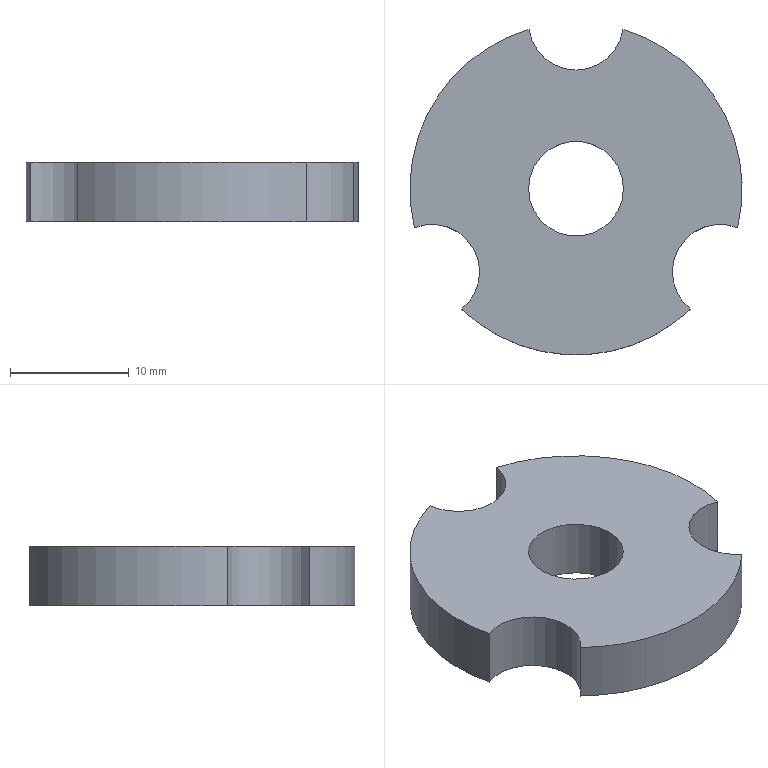Part | STEP file | PN_0002_default | 1 solid | 9 faces | box 28 x 27.429 x 5 mm | volume 2473 mm3 | cylinder 7 | plane 2 | commonest cylinder face diameters 8 x4 28 x3
STEP:
#1=CARTESIAN_POINT('',(0.,0.,0.));
#2=DIRECTION('',(0.,0.,1.));
#3=DIRECTION('',(1.,0.,0.));
#4=AXIS2_PLACEMENT_3D('',#1,#2,#3);
#5=CARTESIAN_POINT('',(-9.65,-10.143,5.));
#6=VERTEX_POINT('',#5);
#7=CARTESIAN_POINT('',(9.65,-10.143,5.));
#8=VERTEX_POINT('',#7);
#9=CARTESIAN_POINT('',(0.,0.,5.));
#10=DIRECTION('',(0.,0.,1.));
#11=DIRECTION('',(1.,0.,0.));
#12=AXIS2_PLACEMENT_3D('',#9,#10,#11);
#13=CIRCLE('',#12,14.);
#14=CARTESIAN_POINT('',(6.062,-3.5,5.));
#15=DIRECTION('',(0.,0.,1.));
#16=DIRECTION('',(1.,0.,0.));
#17=AXIS2_PLACEMENT_3D('',#14,#15,#16);
#18=PLANE('',#17);
#19=CARTESIAN_POINT('',(-6.062,3.5));
#20=DIRECTION('',(1.,0.));
#21=AXIS2_PLACEMENT_2D('',#19,#20);
#22=CIRCLE('',#21,14.);
#23=(GEOMETRIC_REPRESENTATION_CONTEXT(2)PARAMETRIC_REPRESENTATION_CONTEXT()REPRESENTATION_CONTEXT('',''));
#24=DEFINITIONAL_REPRESENTATION('',(#22),#23);
#25=PCURVE('',#18,#24);
#26=CARTESIAN_POINT('',(0.,0.,5.));
#27=DIRECTION('',(0.,0.,-1.));
#28=DIRECTION('',(-1.,0.,0.));
#29=AXIS2_PLACEMENT_3D('',#26,#27,#28);
#30=CYLINDRICAL_SURFACE('',#29,14.);
#31=CARTESIAN_POINT('',(9.425,0.));
#32=DIRECTION('',(-1.,0.));
#33=VECTOR('',#32,1.);
#34=LINE('',#31,#33);
#35=(GEOMETRIC_REPRESENTATION_CONTEXT(2)PARAMETRIC_REPRESENTATION_CONTEXT()REPRESENTATION_CONTEXT('',''));
#36=DEFINITIONAL_REPRESENTATION('',(#34),#35);
#37=PCURVE('',#30,#36);
#38=SURFACE_CURVE('',#13,(#25,#37),.PCURVE_S1.);
#39=EDGE_CURVE('',#6,#8,#38,.T.);
#40=ORIENTED_EDGE('',*,*,#39,.T.);
#41=CARTESIAN_POINT('',(13.609,-3.286,5.));
#42=VERTEX_POINT('',#41);
#43=CARTESIAN_POINT('',(12.124,-7.,5.));
#44=DIRECTION('',(0.,0.,-1.));
#45=DIRECTION('',(1.,0.,0.));
#46=AXIS2_PLACEMENT_3D('',#43,#44,#45);
#47=CIRCLE('',#46,4.);
#48=CARTESIAN_POINT('',(10.062,-3.5));
#49=CARTESIAN_POINT('',(10.062,-10.428));
#50=CARTESIAN_POINT('',(4.062,-6.964));
#51=CARTESIAN_POINT('',(-1.938,-3.5));
#52=CARTESIAN_POINT('',(4.062,-0.0359));
#53=CARTESIAN_POINT('',(10.062,3.428));
#54=CARTESIAN_POINT('',(10.062,-3.5));
#55=(BOUNDED_CURVE()B_SPLINE_CURVE(2,(#48,#49,#50,#51,#52,#53,#54),.UNSPECIFIED.,.T.,.F.)B_SPLINE_CURVE_WITH_KNOTS((1,2,2,2,2,1),(-2.094,0.,2.094,4.189,6.283,8.378),.UNSPECIFIED.)CURVE()GEOMETRIC_REPRESENTATION_ITEM()RATIONAL_B_SPLINE_CURVE((1.,0.5,1.,0.5,1.,0.5,1.))REPRESENTATION_ITEM(''));
#56=(GEOMETRIC_REPRESENTATION_CONTEXT(2)PARAMETRIC_REPRESENTATION_CONTEXT()REPRESENTATION_CONTEXT('',''));
#57=DEFINITIONAL_REPRESENTATION('',(#55),#56);
#58=PCURVE('',#18,#57);
#59=CARTESIAN_POINT('',(12.124,-7.,5.));
#60=DIRECTION('',(0.,0.,-1.));
#61=DIRECTION('',(-1.,0.,0.));
#62=AXIS2_PLACEMENT_3D('',#59,#60,#61);
#63=CYLINDRICAL_SURFACE('',#62,4.);
#64=CARTESIAN_POINT('',(-3.142,0.));
#65=DIRECTION('',(1.,0.));
#66=VECTOR('',#65,1.);
#67=LINE('',#64,#66);
#68=(GEOMETRIC_REPRESENTATION_CONTEXT(2)PARAMETRIC_REPRESENTATION_CONTEXT()REPRESENTATION_CONTEXT('',''));
#69=DEFINITIONAL_REPRESENTATION('',(#67),#68);
#70=PCURVE('',#63,#69);
#71=SURFACE_CURVE('',#47,(#58,#70),.PCURVE_S1.);
#72=EDGE_CURVE('',#8,#42,#71,.T.);
#73=ORIENTED_EDGE('',*,*,#72,.T.);
#74=CARTESIAN_POINT('',(3.959,13.429,5.));
#75=VERTEX_POINT('',#74);
#76=CARTESIAN_POINT('',(0.,0.,5.));
#77=DIRECTION('',(0.,0.,1.));
#78=DIRECTION('',(1.,0.,0.));
#79=AXIS2_PLACEMENT_3D('',#76,#77,#78);
#80=CIRCLE('',#79,14.);
#81=CARTESIAN_POINT('',(-6.062,3.5));
#82=DIRECTION('',(1.,0.));
#83=AXIS2_PLACEMENT_2D('',#81,#82);
#84=CIRCLE('',#83,14.);
#85=(GEOMETRIC_REPRESENTATION_CONTEXT(2)PARAMETRIC_REPRESENTATION_CONTEXT()REPRESENTATION_CONTEXT('',''));
#86=DEFINITIONAL_REPRESENTATION('',(#84),#85);
#87=PCURVE('',#18,#86);
#88=CARTESIAN_POINT('',(0.,0.,5.));
#89=DIRECTION('',(0.,0.,-1.));
#90=DIRECTION('',(-1.,0.,0.));
#91=AXIS2_PLACEMENT_3D('',#88,#89,#90);
#92=CYLINDRICAL_SURFACE('',#91,14.);
#93=CARTESIAN_POINT('',(9.425,0.));
#94=DIRECTION('',(-1.,0.));
#95=VECTOR('',#94,1.);
#96=LINE('',#93,#95);
#97=(GEOMETRIC_REPRESENTATION_CONTEXT(2)PARAMETRIC_REPRESENTATION_CONTEXT()REPRESENTATION_CONTEXT('',''));
#98=DEFINITIONAL_REPRESENTATION('',(#96),#97);
#99=PCURVE('',#92,#98);
#100=SURFACE_CURVE('',#80,(#87,#99),.PCURVE_S1.);
#101=EDGE_CURVE('',#42,#75,#100,.T.);
#102=ORIENTED_EDGE('',*,*,#101,.T.);
#103=CARTESIAN_POINT('',(-3.959,13.429,5.));
#104=VERTEX_POINT('',#103);
#105=CARTESIAN_POINT('',(0.,14.,5.));
#106=DIRECTION('',(0.,0.,-1.));
#107=DIRECTION('',(1.,0.,0.));
#108=AXIS2_PLACEMENT_3D('',#105,#106,#107);
#109=CIRCLE('',#108,4.);
#110=CARTESIAN_POINT('',(-2.062,17.5));
#111=CARTESIAN_POINT('',(-2.062,10.572));
#112=CARTESIAN_POINT('',(-8.062,14.036));
#113=CARTESIAN_POINT('',(-14.062,17.5));
#114=CARTESIAN_POINT('',(-8.062,20.964));
#115=CARTESIAN_POINT('',(-2.062,24.428));
#116=CARTESIAN_POINT('',(-2.062,17.5));
#117=(BOUNDED_CURVE()B_SPLINE_CURVE(2,(#110,#111,#112,#113,#114,#115,#116),.UNSPECIFIED.,.T.,.F.)B_SPLINE_CURVE_WITH_KNOTS((1,2,2,2,2,1),(-2.094,0.,2.094,4.189,6.283,8.378),.UNSPECIFIED.)CURVE()GEOMETRIC_REPRESENTATION_ITEM()RATIONAL_B_SPLINE_CURVE((1.,0.5,1.,0.5,1.,0.5,1.))REPRESENTATION_ITEM(''));
#118=(GEOMETRIC_REPRESENTATION_CONTEXT(2)PARAMETRIC_REPRESENTATION_CONTEXT()REPRESENTATION_CONTEXT('',''));
#119=DEFINITIONAL_REPRESENTATION('',(#117),#118);
#120=PCURVE('',#18,#119);
#121=CARTESIAN_POINT('',(0.,14.,5.));
#122=DIRECTION('',(0.,0.,-1.));
#123=DIRECTION('',(-1.,0.,0.));
#124=AXIS2_PLACEMENT_3D('',#121,#122,#123);
#125=CYLINDRICAL_SURFACE('',#124,4.);
#126=CARTESIAN_POINT('',(3.142,0.));
#127=DIRECTION('',(1.,0.));
#128=VECTOR('',#127,1.);
#129=LINE('',#126,#128);
#130=(GEOMETRIC_REPRESENTATION_CONTEXT(2)PARAMETRIC_REPRESENTATION_CONTEXT()REPRESENTATION_CONTEXT('',''));
#131=DEFINITIONAL_REPRESENTATION('',(#129),#130);
#132=PCURVE('',#125,#131);
#133=SURFACE_CURVE('',#109,(#120,#132),.PCURVE_S1.);
#134=EDGE_CURVE('',#75,#104,#133,.T.);
#135=ORIENTED_EDGE('',*,*,#134,.T.);
#136=CARTESIAN_POINT('',(-13.609,-3.286,5.));
#137=VERTEX_POINT('',#136);
#138=CARTESIAN_POINT('',(0.,0.,5.));
#139=DIRECTION('',(0.,0.,1.));
#140=DIRECTION('',(1.,0.,0.));
#141=AXIS2_PLACEMENT_3D('',#138,#139,#140);
#142=CIRCLE('',#141,14.);
#143=CARTESIAN_POINT('',(-6.062,3.5));
#144=DIRECTION('',(1.,0.));
#145=AXIS2_PLACEMENT_2D('',#143,#144);
#146=CIRCLE('',#145,14.);
#147=(GEOMETRIC_REPRESENTATION_CONTEXT(2)PARAMETRIC_REPRESENTATION_CONTEXT()REPRESENTATION_CONTEXT('',''));
#148=DEFINITIONAL_REPRESENTATION('',(#146),#147);
#149=PCURVE('',#18,#148);
#150=CARTESIAN_POINT('',(0.,0.,5.));
#151=DIRECTION('',(0.,0.,-1.));
#152=DIRECTION('',(-1.,0.,0.));
#153=AXIS2_PLACEMENT_3D('',#150,#151,#152);
#154=CYLINDRICAL_SURFACE('',#153,14.);
#155=CARTESIAN_POINT('',(3.142,0.));
#156=DIRECTION('',(-1.,0.));
#157=VECTOR('',#156,1.);
#158=LINE('',#155,#157);
#159=(GEOMETRIC_REPRESENTATION_CONTEXT(2)PARAMETRIC_REPRESENTATION_CONTEXT()REPRESENTATION_CONTEXT('',''));
#160=DEFINITIONAL_REPRESENTATION('',(#158),#159);
#161=PCURVE('',#154,#160);
#162=SURFACE_CURVE('',#142,(#149,#161),.PCURVE_S1.);
#163=EDGE_CURVE('',#104,#137,#162,.T.);
#164=ORIENTED_EDGE('',*,*,#163,.T.);
#165=CARTESIAN_POINT('',(-12.124,-7.,5.));
#166=DIRECTION('',(0.,0.,-1.));
#167=DIRECTION('',(1.,0.,0.));
#168=AXIS2_PLACEMENT_3D('',#165,#166,#167);
#169=CIRCLE('',#168,4.);
#170=CARTESIAN_POINT('',(-14.187,-3.5));
#171=CARTESIAN_POINT('',(-14.187,-10.428));
#172=CARTESIAN_POINT('',(-20.187,-6.964));
#173=CARTESIAN_POINT('',(-26.187,-3.5));
#174=CARTESIAN_POINT('',(-20.187,-0.0359));
#175=CARTESIAN_POINT('',(-14.187,3.428));
#176=CARTESIAN_POINT('',(-14.187,-3.5));
#177=(BOUNDED_CURVE()B_SPLINE_CURVE(2,(#170,#171,#172,#173,#174,#175,#176),.UNSPECIFIED.,.T.,.F.)B_SPLINE_CURVE_WITH_KNOTS((1,2,2,2,2,1),(-2.094,0.,2.094,4.189,6.283,8.378),.UNSPECIFIED.)CURVE()GEOMETRIC_REPRESENTATION_ITEM()RATIONAL_B_SPLINE_CURVE((1.,0.5,1.,0.5,1.,0.5,1.))REPRESENTATION_ITEM(''));
#178=(GEOMETRIC_REPRESENTATION_CONTEXT(2)PARAMETRIC_REPRESENTATION_CONTEXT()REPRESENTATION_CONTEXT('',''));
#179=DEFINITIONAL_REPRESENTATION('',(#177),#178);
#180=PCURVE('',#18,#179);
#181=CARTESIAN_POINT('',(-12.124,-7.,5.));
#182=DIRECTION('',(0.,0.,-1.));
#183=DIRECTION('',(-1.,0.,0.));
#184=AXIS2_PLACEMENT_3D('',#181,#182,#183);
#185=CYLINDRICAL_SURFACE('',#184,4.);
#186=CARTESIAN_POINT('',(-3.142,0.));
#187=DIRECTION('',(1.,0.));
#188=VECTOR('',#187,1.);
#189=LINE('',#186,#188);
#190=(GEOMETRIC_REPRESENTATION_CONTEXT(2)PARAMETRIC_REPRESENTATION_CONTEXT()REPRESENTATION_CONTEXT('',''));
#191=DEFINITIONAL_REPRESENTATION('',(#189),#190);
#192=PCURVE('',#185,#191);
#193=SURFACE_CURVE('',#169,(#180,#192),.PCURVE_S1.);
#194=EDGE_CURVE('',#137,#6,#193,.T.);
#195=ORIENTED_EDGE('',*,*,#194,.T.);
#196=EDGE_LOOP('',(#40,#73,#102,#135,#164,#195));
#197=FACE_BOUND('',#196,.T.);
#198=CARTESIAN_POINT('',(4.,0.,5.));
#199=VERTEX_POINT('',#198);
#200=CARTESIAN_POINT('',(0.,0.,5.));
#201=DIRECTION('',(0.,0.,1.));
#202=DIRECTION('',(1.,0.,0.));
#203=AXIS2_PLACEMENT_3D('',#200,#201,#202);
#204=CIRCLE('',#203,4.);
#205=CARTESIAN_POINT('',(-6.062,3.5));
#206=DIRECTION('',(1.,0.));
#207=AXIS2_PLACEMENT_2D('',#205,#206);
#208=CIRCLE('',#207,4.);
#209=(GEOMETRIC_REPRESENTATION_CONTEXT(2)PARAMETRIC_REPRESENTATION_CONTEXT()REPRESENTATION_CONTEXT('',''));
#210=DEFINITIONAL_REPRESENTATION('',(#208),#209);
#211=PCURVE('',#18,#210);
#212=CARTESIAN_POINT('',(0.,0.,5.));
#213=DIRECTION('',(0.,0.,-1.));
#214=DIRECTION('',(-1.,0.,0.));
#215=AXIS2_PLACEMENT_3D('',#212,#213,#214);
#216=CYLINDRICAL_SURFACE('',#215,4.);
#217=CARTESIAN_POINT('',(9.425,0.));
#218=DIRECTION('',(-1.,0.));
#219=VECTOR('',#218,1.);
#220=LINE('',#217,#219);
#221=(GEOMETRIC_REPRESENTATION_CONTEXT(2)PARAMETRIC_REPRESENTATION_CONTEXT()REPRESENTATION_CONTEXT('',''));
#222=DEFINITIONAL_REPRESENTATION('',(#220),#221);
#223=PCURVE('',#216,#222);
#224=SURFACE_CURVE('',#204,(#211,#223),.PCURVE_S1.);
#225=EDGE_CURVE('',#199,#199,#224,.T.);
#226=ORIENTED_EDGE('',*,*,#225,.F.);
#227=EDGE_LOOP('',(#226));
#228=FACE_BOUND('',#227,.T.);
#229=ADVANCED_FACE('',(#197,#228),#18,.T.);
#230=CARTESIAN_POINT('',(-9.65,-10.143,0.));
#231=VERTEX_POINT('',#230);
#232=CARTESIAN_POINT('',(9.65,-10.143,0.));
#233=VERTEX_POINT('',#232);
#234=CARTESIAN_POINT('',(0.,0.,0.));
#235=DIRECTION('',(0.,0.,1.));
#236=DIRECTION('',(1.,0.,0.));
#237=AXIS2_PLACEMENT_3D('',#234,#235,#236);
#238=CIRCLE('',#237,14.);
#239=CARTESIAN_POINT('',(6.062,-3.5,0.));
#240=DIRECTION('',(0.,0.,1.));
#241=DIRECTION('',(1.,0.,0.));
#242=AXIS2_PLACEMENT_3D('',#239,#240,#241);
#243=PLANE('',#242);
#244=CARTESIAN_POINT('',(-6.062,3.5));
#245=DIRECTION('',(1.,0.));
#246=AXIS2_PLACEMENT_2D('',#244,#245);
#247=CIRCLE('',#246,14.);
#248=(GEOMETRIC_REPRESENTATION_CONTEXT(2)PARAMETRIC_REPRESENTATION_CONTEXT()REPRESENTATION_CONTEXT('',''));
#249=DEFINITIONAL_REPRESENTATION('',(#247),#248);
#250=PCURVE('',#243,#249);
#251=CARTESIAN_POINT('',(9.425,5.));
#252=DIRECTION('',(-1.,0.));
#253=VECTOR('',#252,1.);
#254=LINE('',#251,#253);
#255=(GEOMETRIC_REPRESENTATION_CONTEXT(2)PARAMETRIC_REPRESENTATION_CONTEXT()REPRESENTATION_CONTEXT('',''));
#256=DEFINITIONAL_REPRESENTATION('',(#254),#255);
#257=PCURVE('',#30,#256);
#258=SURFACE_CURVE('',#238,(#250,#257),.PCURVE_S1.);
#259=EDGE_CURVE('',#231,#233,#258,.T.);
#260=ORIENTED_EDGE('',*,*,#259,.F.);
#261=CARTESIAN_POINT('',(-13.609,-3.286,0.));
#262=VERTEX_POINT('',#261);
#263=CARTESIAN_POINT('',(-12.124,-7.,0.));
#264=DIRECTION('',(0.,0.,-1.));
#265=DIRECTION('',(1.,0.,0.));
#266=AXIS2_PLACEMENT_3D('',#263,#264,#265);
#267=CIRCLE('',#266,4.);
#268=CARTESIAN_POINT('',(-14.187,-3.5));
#269=CARTESIAN_POINT('',(-14.187,-10.428));
#270=CARTESIAN_POINT('',(-20.187,-6.964));
#271=CARTESIAN_POINT('',(-26.187,-3.5));
#272=CARTESIAN_POINT('',(-20.187,-0.0359));
#273=CARTESIAN_POINT('',(-14.187,3.428));
#274=CARTESIAN_POINT('',(-14.187,-3.5));
#275=(BOUNDED_CURVE()B_SPLINE_CURVE(2,(#268,#269,#270,#271,#272,#273,#274),.UNSPECIFIED.,.T.,.F.)B_SPLINE_CURVE_WITH_KNOTS((1,2,2,2,2,1),(-2.094,0.,2.094,4.189,6.283,8.378),.UNSPECIFIED.)CURVE()GEOMETRIC_REPRESENTATION_ITEM()RATIONAL_B_SPLINE_CURVE((1.,0.5,1.,0.5,1.,0.5,1.))REPRESENTATION_ITEM(''));
#276=(GEOMETRIC_REPRESENTATION_CONTEXT(2)PARAMETRIC_REPRESENTATION_CONTEXT()REPRESENTATION_CONTEXT('',''));
#277=DEFINITIONAL_REPRESENTATION('',(#275),#276);
#278=PCURVE('',#243,#277);
#279=CARTESIAN_POINT('',(-3.142,5.));
#280=DIRECTION('',(1.,0.));
#281=VECTOR('',#280,1.);
#282=LINE('',#279,#281);
#283=(GEOMETRIC_REPRESENTATION_CONTEXT(2)PARAMETRIC_REPRESENTATION_CONTEXT()REPRESENTATION_CONTEXT('',''));
#284=DEFINITIONAL_REPRESENTATION('',(#282),#283);
#285=PCURVE('',#185,#284);
#286=SURFACE_CURVE('',#267,(#278,#285),.PCURVE_S1.);
#287=EDGE_CURVE('',#262,#231,#286,.T.);
#288=ORIENTED_EDGE('',*,*,#287,.F.);
#289=CARTESIAN_POINT('',(-3.959,13.429,0.));
#290=VERTEX_POINT('',#289);
#291=CARTESIAN_POINT('',(0.,0.,0.));
#292=DIRECTION('',(0.,0.,1.));
#293=DIRECTION('',(1.,0.,0.));
#294=AXIS2_PLACEMENT_3D('',#291,#292,#293);
#295=CIRCLE('',#294,14.);
#296=CARTESIAN_POINT('',(-6.062,3.5));
#297=DIRECTION('',(1.,0.));
#298=AXIS2_PLACEMENT_2D('',#296,#297);
#299=CIRCLE('',#298,14.);
#300=(GEOMETRIC_REPRESENTATION_CONTEXT(2)PARAMETRIC_REPRESENTATION_CONTEXT()REPRESENTATION_CONTEXT('',''));
#301=DEFINITIONAL_REPRESENTATION('',(#299),#300);
#302=PCURVE('',#243,#301);
#303=CARTESIAN_POINT('',(3.142,5.));
#304=DIRECTION('',(-1.,0.));
#305=VECTOR('',#304,1.);
#306=LINE('',#303,#305);
#307=(GEOMETRIC_REPRESENTATION_CONTEXT(2)PARAMETRIC_REPRESENTATION_CONTEXT()REPRESENTATION_CONTEXT('',''));
#308=DEFINITIONAL_REPRESENTATION('',(#306),#307);
#309=PCURVE('',#154,#308);
#310=SURFACE_CURVE('',#295,(#302,#309),.PCURVE_S1.);
#311=EDGE_CURVE('',#290,#262,#310,.T.);
#312=ORIENTED_EDGE('',*,*,#311,.F.);
#313=CARTESIAN_POINT('',(3.959,13.429,0.));
#314=VERTEX_POINT('',#313);
#315=CARTESIAN_POINT('',(0.,14.,0.));
#316=DIRECTION('',(0.,0.,-1.));
#317=DIRECTION('',(1.,0.,0.));
#318=AXIS2_PLACEMENT_3D('',#315,#316,#317);
#319=CIRCLE('',#318,4.);
#320=CARTESIAN_POINT('',(-2.062,17.5));
#321=CARTESIAN_POINT('',(-2.062,10.572));
#322=CARTESIAN_POINT('',(-8.062,14.036));
#323=CARTESIAN_POINT('',(-14.062,17.5));
#324=CARTESIAN_POINT('',(-8.062,20.964));
#325=CARTESIAN_POINT('',(-2.062,24.428));
#326=CARTESIAN_POINT('',(-2.062,17.5));
#327=(BOUNDED_CURVE()B_SPLINE_CURVE(2,(#320,#321,#322,#323,#324,#325,#326),.UNSPECIFIED.,.T.,.F.)B_SPLINE_CURVE_WITH_KNOTS((1,2,2,2,2,1),(-2.094,0.,2.094,4.189,6.283,8.378),.UNSPECIFIED.)CURVE()GEOMETRIC_REPRESENTATION_ITEM()RATIONAL_B_SPLINE_CURVE((1.,0.5,1.,0.5,1.,0.5,1.))REPRESENTATION_ITEM(''));
#328=(GEOMETRIC_REPRESENTATION_CONTEXT(2)PARAMETRIC_REPRESENTATION_CONTEXT()REPRESENTATION_CONTEXT('',''));
#329=DEFINITIONAL_REPRESENTATION('',(#327),#328);
#330=PCURVE('',#243,#329);
#331=CARTESIAN_POINT('',(3.142,5.));
#332=DIRECTION('',(1.,0.));
#333=VECTOR('',#332,1.);
#334=LINE('',#331,#333);
#335=(GEOMETRIC_REPRESENTATION_CONTEXT(2)PARAMETRIC_REPRESENTATION_CONTEXT()REPRESENTATION_CONTEXT('',''));
#336=DEFINITIONAL_REPRESENTATION('',(#334),#335);
#337=PCURVE('',#125,#336);
#338=SURFACE_CURVE('',#319,(#330,#337),.PCURVE_S1.);
#339=EDGE_CURVE('',#314,#290,#338,.T.);
#340=ORIENTED_EDGE('',*,*,#339,.F.);
#341=CARTESIAN_POINT('',(13.609,-3.286,0.));
#342=VERTEX_POINT('',#341);
#343=CARTESIAN_POINT('',(0.,0.,0.));
#344=DIRECTION('',(0.,0.,1.));
#345=DIRECTION('',(1.,0.,0.));
#346=AXIS2_PLACEMENT_3D('',#343,#344,#345);
#347=CIRCLE('',#346,14.);
#348=CARTESIAN_POINT('',(-6.062,3.5));
#349=DIRECTION('',(1.,0.));
#350=AXIS2_PLACEMENT_2D('',#348,#349);
#351=CIRCLE('',#350,14.);
#352=(GEOMETRIC_REPRESENTATION_CONTEXT(2)PARAMETRIC_REPRESENTATION_CONTEXT()REPRESENTATION_CONTEXT('',''));
#353=DEFINITIONAL_REPRESENTATION('',(#351),#352);
#354=PCURVE('',#243,#353);
#355=CARTESIAN_POINT('',(9.425,5.));
#356=DIRECTION('',(-1.,0.));
#357=VECTOR('',#356,1.);
#358=LINE('',#355,#357);
#359=(GEOMETRIC_REPRESENTATION_CONTEXT(2)PARAMETRIC_REPRESENTATION_CONTEXT()REPRESENTATION_CONTEXT('',''));
#360=DEFINITIONAL_REPRESENTATION('',(#358),#359);
#361=PCURVE('',#92,#360);
#362=SURFACE_CURVE('',#347,(#354,#361),.PCURVE_S1.);
#363=EDGE_CURVE('',#342,#314,#362,.T.);
#364=ORIENTED_EDGE('',*,*,#363,.F.);
#365=CARTESIAN_POINT('',(12.124,-7.,0.));
#366=DIRECTION('',(0.,0.,-1.));
#367=DIRECTION('',(1.,0.,0.));
#368=AXIS2_PLACEMENT_3D('',#365,#366,#367);
#369=CIRCLE('',#368,4.);
#370=CARTESIAN_POINT('',(10.062,-3.5));
#371=CARTESIAN_POINT('',(10.062,-10.428));
#372=CARTESIAN_POINT('',(4.062,-6.964));
#373=CARTESIAN_POINT('',(-1.938,-3.5));
#374=CARTESIAN_POINT('',(4.062,-0.0359));
#375=CARTESIAN_POINT('',(10.062,3.428));
#376=CARTESIAN_POINT('',(10.062,-3.5));
#377=(BOUNDED_CURVE()B_SPLINE_CURVE(2,(#370,#371,#372,#373,#374,#375,#376),.UNSPECIFIED.,.T.,.F.)B_SPLINE_CURVE_WITH_KNOTS((1,2,2,2,2,1),(-2.094,0.,2.094,4.189,6.283,8.378),.UNSPECIFIED.)CURVE()GEOMETRIC_REPRESENTATION_ITEM()RATIONAL_B_SPLINE_CURVE((1.,0.5,1.,0.5,1.,0.5,1.))REPRESENTATION_ITEM(''));
#378=(GEOMETRIC_REPRESENTATION_CONTEXT(2)PARAMETRIC_REPRESENTATION_CONTEXT()REPRESENTATION_CONTEXT('',''));
#379=DEFINITIONAL_REPRESENTATION('',(#377),#378);
#380=PCURVE('',#243,#379);
#381=CARTESIAN_POINT('',(-3.142,5.));
#382=DIRECTION('',(1.,0.));
#383=VECTOR('',#382,1.);
#384=LINE('',#381,#383);
#385=(GEOMETRIC_REPRESENTATION_CONTEXT(2)PARAMETRIC_REPRESENTATION_CONTEXT()REPRESENTATION_CONTEXT('',''));
#386=DEFINITIONAL_REPRESENTATION('',(#384),#385);
#387=PCURVE('',#63,#386);
#388=SURFACE_CURVE('',#369,(#380,#387),.PCURVE_S1.);
#389=EDGE_CURVE('',#233,#342,#388,.T.);
#390=ORIENTED_EDGE('',*,*,#389,.F.);
#391=EDGE_LOOP('',(#260,#288,#312,#340,#364,#390));
#392=FACE_BOUND('',#391,.T.);
#393=CARTESIAN_POINT('',(4.,0.,0.));
#394=VERTEX_POINT('',#393);
#395=CARTESIAN_POINT('',(0.,0.,0.));
#396=DIRECTION('',(0.,0.,1.));
#397=DIRECTION('',(1.,0.,0.));
#398=AXIS2_PLACEMENT_3D('',#395,#396,#397);
#399=CIRCLE('',#398,4.);
#400=CARTESIAN_POINT('',(-6.062,3.5));
#401=DIRECTION('',(1.,0.));
#402=AXIS2_PLACEMENT_2D('',#400,#401);
#403=CIRCLE('',#402,4.);
#404=(GEOMETRIC_REPRESENTATION_CONTEXT(2)PARAMETRIC_REPRESENTATION_CONTEXT()REPRESENTATION_CONTEXT('',''));
#405=DEFINITIONAL_REPRESENTATION('',(#403),#404);
#406=PCURVE('',#243,#405);
#407=CARTESIAN_POINT('',(9.425,5.));
#408=DIRECTION('',(-1.,0.));
#409=VECTOR('',#408,1.);
#410=LINE('',#407,#409);
#411=(GEOMETRIC_REPRESENTATION_CONTEXT(2)PARAMETRIC_REPRESENTATION_CONTEXT()REPRESENTATION_CONTEXT('',''));
#412=DEFINITIONAL_REPRESENTATION('',(#410),#411);
#413=PCURVE('',#216,#412);
#414=SURFACE_CURVE('',#399,(#406,#413),.PCURVE_S1.);
#415=EDGE_CURVE('',#394,#394,#414,.T.);
#416=ORIENTED_EDGE('',*,*,#415,.T.);
#417=EDGE_LOOP('',(#416));
#418=FACE_BOUND('',#417,.T.);
#419=ADVANCED_FACE('',(#392,#418),#243,.F.);
#420=ORIENTED_EDGE('',*,*,#259,.T.);
#421=CARTESIAN_POINT('',(9.65,-10.143,5.));
#422=DIRECTION('',(0.,0.,-1.));
#423=VECTOR('',#422,1.);
#424=LINE('',#421,#423);
#425=CARTESIAN_POINT('',(3.952,0.));
#426=DIRECTION('',(0.,1.));
#427=VECTOR('',#426,1.);
#428=LINE('',#425,#427);
#429=(GEOMETRIC_REPRESENTATION_CONTEXT(2)PARAMETRIC_REPRESENTATION_CONTEXT()REPRESENTATION_CONTEXT('',''));
#430=DEFINITIONAL_REPRESENTATION('',(#428),#429);
#431=PCURVE('',#30,#430);
#432=CARTESIAN_POINT('',(-0.9038,0.));
#433=DIRECTION('',(0.,1.));
#434=VECTOR('',#433,1.);
#435=LINE('',#432,#434);
#436=(GEOMETRIC_REPRESENTATION_CONTEXT(2)PARAMETRIC_REPRESENTATION_CONTEXT()REPRESENTATION_CONTEXT('',''));
#437=DEFINITIONAL_REPRESENTATION('',(#435),#436);
#438=PCURVE('',#63,#437);
#439=SURFACE_CURVE('',#424,(#431,#438),.PCURVE_S1.);
#440=EDGE_CURVE('',#8,#233,#439,.T.);
#441=ORIENTED_EDGE('',*,*,#440,.F.);
#442=ORIENTED_EDGE('',*,*,#39,.F.);
#443=CARTESIAN_POINT('',(-9.65,-10.143,5.));
#444=DIRECTION('',(0.,0.,-1.));
#445=VECTOR('',#444,1.);
#446=LINE('',#443,#445);
#447=CARTESIAN_POINT('',(5.473,0.));
#448=DIRECTION('',(0.,1.));
#449=VECTOR('',#448,1.);
#450=LINE('',#447,#449);
#451=(GEOMETRIC_REPRESENTATION_CONTEXT(2)PARAMETRIC_REPRESENTATION_CONTEXT()REPRESENTATION_CONTEXT('',''));
#452=DEFINITIONAL_REPRESENTATION('',(#450),#451);
#453=PCURVE('',#30,#452);
#454=CARTESIAN_POINT('',(4.045,0.));
#455=DIRECTION('',(0.,1.));
#456=VECTOR('',#455,1.);
#457=LINE('',#454,#456);
#458=(GEOMETRIC_REPRESENTATION_CONTEXT(2)PARAMETRIC_REPRESENTATION_CONTEXT()REPRESENTATION_CONTEXT('',''));
#459=DEFINITIONAL_REPRESENTATION('',(#457),#458);
#460=PCURVE('',#185,#459);
#461=SURFACE_CURVE('',#446,(#453,#460),.PCURVE_S1.);
#462=EDGE_CURVE('',#6,#231,#461,.T.);
#463=ORIENTED_EDGE('',*,*,#462,.T.);
#464=EDGE_LOOP('',(#420,#441,#442,#463));
#465=FACE_BOUND('',#464,.T.);
#466=ADVANCED_FACE('',(#465),#30,.T.);
#467=ORIENTED_EDGE('',*,*,#440,.F.);
#468=ORIENTED_EDGE('',*,*,#72,.T.);
#469=CARTESIAN_POINT('',(13.609,-3.286,5.));
#470=DIRECTION('',(0.,0.,-1.));
#471=VECTOR('',#470,1.);
#472=LINE('',#469,#471);
#473=CARTESIAN_POINT('',(1.951,0.));
#474=DIRECTION('',(0.,1.));
#475=VECTOR('',#474,1.);
#476=LINE('',#473,#475);
#477=(GEOMETRIC_REPRESENTATION_CONTEXT(2)PARAMETRIC_REPRESENTATION_CONTEXT()REPRESENTATION_CONTEXT('',''));
#478=DEFINITIONAL_REPRESENTATION('',(#476),#477);
#479=PCURVE('',#63,#478);
#480=CARTESIAN_POINT('',(3.378,0.));
#481=DIRECTION('',(0.,1.));
#482=VECTOR('',#481,1.);
#483=LINE('',#480,#482);
#484=(GEOMETRIC_REPRESENTATION_CONTEXT(2)PARAMETRIC_REPRESENTATION_CONTEXT()REPRESENTATION_CONTEXT('',''));
#485=DEFINITIONAL_REPRESENTATION('',(#483),#484);
#486=PCURVE('',#92,#485);
#487=SURFACE_CURVE('',#472,(#479,#486),.PCURVE_S1.);
#488=EDGE_CURVE('',#42,#342,#487,.T.);
#489=ORIENTED_EDGE('',*,*,#488,.T.);
#490=ORIENTED_EDGE('',*,*,#389,.F.);
#491=EDGE_LOOP('',(#467,#468,#489,#490));
#492=FACE_BOUND('',#491,.F.);
#493=ADVANCED_FACE('',(#492),#63,.F.);
#494=ORIENTED_EDGE('',*,*,#363,.T.);
#495=CARTESIAN_POINT('',(3.959,13.429,5.));
#496=DIRECTION('',(0.,0.,-1.));
#497=VECTOR('',#496,1.);
#498=LINE('',#495,#497);
#499=CARTESIAN_POINT('',(1.857,0.));
#500=DIRECTION('',(0.,1.));
#501=VECTOR('',#500,1.);
#502=LINE('',#499,#501);
#503=(GEOMETRIC_REPRESENTATION_CONTEXT(2)PARAMETRIC_REPRESENTATION_CONTEXT()REPRESENTATION_CONTEXT('',''));
#504=DEFINITIONAL_REPRESENTATION('',(#502),#503);
#505=PCURVE('',#92,#504);
#506=CARTESIAN_POINT('',(3.285,0.));
#507=DIRECTION('',(0.,1.));
#508=VECTOR('',#507,1.);
#509=LINE('',#506,#508);
#510=(GEOMETRIC_REPRESENTATION_CONTEXT(2)PARAMETRIC_REPRESENTATION_CONTEXT()REPRESENTATION_CONTEXT('',''));
#511=DEFINITIONAL_REPRESENTATION('',(#509),#510);
#512=PCURVE('',#125,#511);
#513=SURFACE_CURVE('',#498,(#505,#512),.PCURVE_S1.);
#514=EDGE_CURVE('',#75,#314,#513,.T.);
#515=ORIENTED_EDGE('',*,*,#514,.F.);
#516=ORIENTED_EDGE('',*,*,#101,.F.);
#517=ORIENTED_EDGE('',*,*,#488,.T.);
#518=EDGE_LOOP('',(#494,#515,#516,#517));
#519=FACE_BOUND('',#518,.T.);
#520=ADVANCED_FACE('',(#519),#92,.T.);
#521=ORIENTED_EDGE('',*,*,#514,.F.);
#522=ORIENTED_EDGE('',*,*,#134,.T.);
#523=CARTESIAN_POINT('',(-3.959,13.429,5.));
#524=DIRECTION('',(0.,0.,-1.));
#525=VECTOR('',#524,1.);
#526=LINE('',#523,#525);
#527=CARTESIAN_POINT('',(6.14,0.));
#528=DIRECTION('',(0.,1.));
#529=VECTOR('',#528,1.);
#530=LINE('',#527,#529);
#531=(GEOMETRIC_REPRESENTATION_CONTEXT(2)PARAMETRIC_REPRESENTATION_CONTEXT()REPRESENTATION_CONTEXT('',''));
#532=DEFINITIONAL_REPRESENTATION('',(#530),#531);
#533=PCURVE('',#125,#532);
#534=CARTESIAN_POINT('',(1.284,0.));
#535=DIRECTION('',(0.,1.));
#536=VECTOR('',#535,1.);
#537=LINE('',#534,#536);
#538=(GEOMETRIC_REPRESENTATION_CONTEXT(2)PARAMETRIC_REPRESENTATION_CONTEXT()REPRESENTATION_CONTEXT('',''));
#539=DEFINITIONAL_REPRESENTATION('',(#537),#538);
#540=PCURVE('',#154,#539);
#541=SURFACE_CURVE('',#526,(#533,#540),.PCURVE_S1.);
#542=EDGE_CURVE('',#104,#290,#541,.T.);
#543=ORIENTED_EDGE('',*,*,#542,.T.);
#544=ORIENTED_EDGE('',*,*,#339,.F.);
#545=EDGE_LOOP('',(#521,#522,#543,#544));
#546=FACE_BOUND('',#545,.F.);
#547=ADVANCED_FACE('',(#546),#125,.F.);
#548=ORIENTED_EDGE('',*,*,#311,.T.);
#549=CARTESIAN_POINT('',(-13.609,-3.286,5.));
#550=DIRECTION('',(0.,0.,-1.));
#551=VECTOR('',#550,1.);
#552=LINE('',#549,#551);
#553=CARTESIAN_POINT('',(-0.2369,0.));
#554=DIRECTION('',(0.,1.));
#555=VECTOR('',#554,1.);
#556=LINE('',#553,#555);
#557=(GEOMETRIC_REPRESENTATION_CONTEXT(2)PARAMETRIC_REPRESENTATION_CONTEXT()REPRESENTATION_CONTEXT('',''));
#558=DEFINITIONAL_REPRESENTATION('',(#556),#557);
#559=PCURVE('',#154,#558);
#560=CARTESIAN_POINT('',(1.191,0.));
#561=DIRECTION('',(0.,1.));
#562=VECTOR('',#561,1.);
#563=LINE('',#560,#562);
#564=(GEOMETRIC_REPRESENTATION_CONTEXT(2)PARAMETRIC_REPRESENTATION_CONTEXT()REPRESENTATION_CONTEXT('',''));
#565=DEFINITIONAL_REPRESENTATION('',(#563),#564);
#566=PCURVE('',#185,#565);
#567=SURFACE_CURVE('',#552,(#559,#566),.PCURVE_S1.);
#568=EDGE_CURVE('',#137,#262,#567,.T.);
#569=ORIENTED_EDGE('',*,*,#568,.F.);
#570=ORIENTED_EDGE('',*,*,#163,.F.);
#571=ORIENTED_EDGE('',*,*,#542,.T.);
#572=EDGE_LOOP('',(#548,#569,#570,#571));
#573=FACE_BOUND('',#572,.T.);
#574=ADVANCED_FACE('',(#573),#154,.T.);
#575=ORIENTED_EDGE('',*,*,#568,.F.);
#576=ORIENTED_EDGE('',*,*,#194,.T.);
#577=ORIENTED_EDGE('',*,*,#462,.T.);
#578=ORIENTED_EDGE('',*,*,#287,.F.);
#579=EDGE_LOOP('',(#575,#576,#577,#578));
#580=FACE_BOUND('',#579,.F.);
#581=ADVANCED_FACE('',(#580),#185,.F.);
#582=ORIENTED_EDGE('',*,*,#225,.F.);
#583=CARTESIAN_POINT('',(4.,0.,5.));
#584=CARTESIAN_POINT('',(4.,0.,0.));
#585=B_SPLINE_CURVE_WITH_KNOTS('',1,(#583,#584),.UNSPECIFIED.,.F.,.F.,(2,2),(0.,5.),.PIECEWISE_BEZIER_KNOTS.);
#586=CARTESIAN_POINT('',(9.425,0.));
#587=DIRECTION('',(0.,1.));
#588=VECTOR('',#587,1.);
#589=LINE('',#586,#588);
#590=(GEOMETRIC_REPRESENTATION_CONTEXT(2)PARAMETRIC_REPRESENTATION_CONTEXT()REPRESENTATION_CONTEXT('',''));
#591=DEFINITIONAL_REPRESENTATION('',(#589),#590);
#592=PCURVE('',#216,#591);
#593=CARTESIAN_POINT('',(3.142,0.));
#594=DIRECTION('',(0.,1.));
#595=VECTOR('',#594,1.);
#596=LINE('',#593,#595);
#597=(GEOMETRIC_REPRESENTATION_CONTEXT(2)PARAMETRIC_REPRESENTATION_CONTEXT()REPRESENTATION_CONTEXT('',''));
#598=DEFINITIONAL_REPRESENTATION('',(#596),#597);
#599=PCURVE('',#216,#598);
#600=SEAM_CURVE('',#585,(#592,#599),.PCURVE_S1.);
#601=EDGE_CURVE('',#199,#394,#600,.T.);
#602=ORIENTED_EDGE('',*,*,#601,.T.);
#603=ORIENTED_EDGE('',*,*,#415,.T.);
#604=ORIENTED_EDGE('',*,*,#601,.F.);
#605=EDGE_LOOP('',(#582,#602,#603,#604));
#606=FACE_BOUND('',#605,.F.);
#607=ADVANCED_FACE('',(#606),#216,.F.);
#608=CLOSED_SHELL('',(#229,#419,#466,#493,#520,#547,#574,#581,#607));
#609=MANIFOLD_SOLID_BREP('',#608);
#610=(LENGTH_UNIT()NAMED_UNIT(*)SI_UNIT(.MILLI.,.METRE.));
#611=UNCERTAINTY_MEASURE_WITH_UNIT(LENGTH_MEASURE(0.000001),#610,'','');
#612=(NAMED_UNIT(*)PLANE_ANGLE_UNIT()SI_UNIT($,.RADIAN.));
#613=(NAMED_UNIT(*)SI_UNIT($,.STERADIAN.)SOLID_ANGLE_UNIT());
#614=(GEOMETRIC_REPRESENTATION_CONTEXT(3)GLOBAL_UNCERTAINTY_ASSIGNED_CONTEXT((#611))GLOBAL_UNIT_ASSIGNED_CONTEXT((#610,#612,#613))REPRESENTATION_CONTEXT('',''));
#615=ADVANCED_BREP_SHAPE_REPRESENTATION('',(#4,#609),#614);